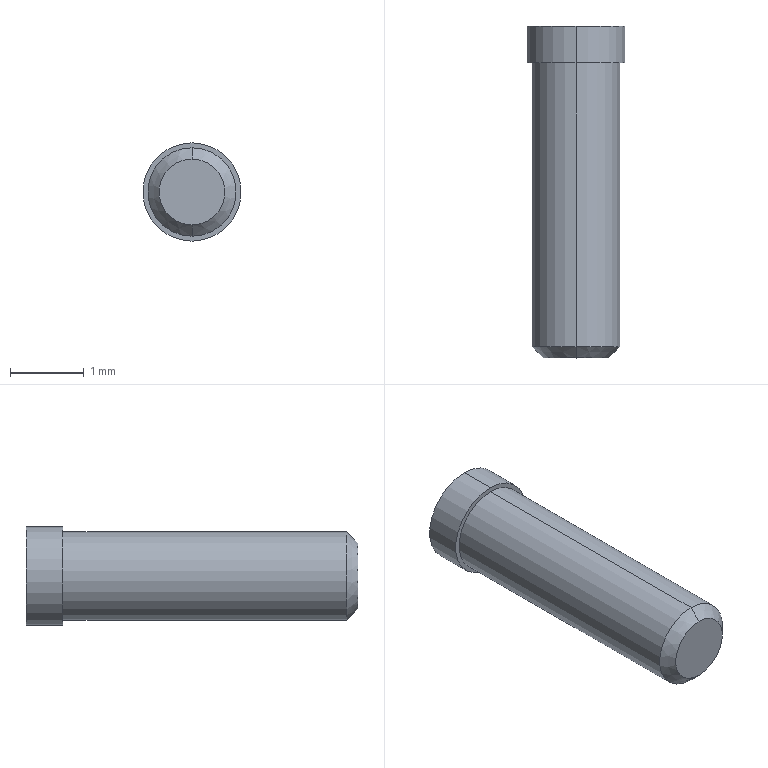Part | STEP file | MG_Plug_Screw_9_N | 1 solid | 16 faces | box 1.333 x 4.5 x 1.333 mm | volume 5.052 mm3 | plane 10 | cylinder 4 | cone 2 | commonest cylinder face diameters 1.2 x2 1.333 x2
STEP:
#1=CARTESIAN_POINT('',(0.,0.,0.));
#2=DIRECTION('',(0.,0.,1.));
#3=DIRECTION('',(1.,0.,0.));
#4=AXIS2_PLACEMENT_3D('',#1,#2,#3);
#5=CARTESIAN_POINT('',(0.,-4.,0.4465));
#6=VERTEX_POINT('',#5);
#7=CARTESIAN_POINT('',(0.,-4.,-0.4465));
#8=VERTEX_POINT('',#7);
#9=CARTESIAN_POINT('',(0.,-4.,0.));
#10=DIRECTION('',(0.,1.,0.));
#11=DIRECTION('',(0.,0.,1.));
#12=AXIS2_PLACEMENT_3D('',#9,#10,#11);
#13=CIRCLE('',#12,0.4465);
#14=CARTESIAN_POINT('',(0.,-4.,0.));
#15=DIRECTION('',(0.,1.,0.));
#16=DIRECTION('',(0.,0.,1.));
#17=AXIS2_PLACEMENT_3D('',#14,#15,#16);
#18=CONICAL_SURFACE('',#17,0.4465,0.7854);
#19=CARTESIAN_POINT('',(0.,0.));
#20=DIRECTION('',(1.,0.));
#21=VECTOR('',#20,1.);
#22=LINE('',#19,#21);
#23=(GEOMETRIC_REPRESENTATION_CONTEXT(2)PARAMETRIC_REPRESENTATION_CONTEXT()REPRESENTATION_CONTEXT('',''));
#24=DEFINITIONAL_REPRESENTATION('',(#22),#23);
#25=PCURVE('',#18,#24);
#26=CARTESIAN_POINT('',(0.4465,-4.,0.));
#27=DIRECTION('',(0.,1.,0.));
#28=DIRECTION('',(0.,0.,1.));
#29=AXIS2_PLACEMENT_3D('',#26,#27,#28);
#30=PLANE('',#29);
#31=CARTESIAN_POINT('',(0.,-0.4465));
#32=DIRECTION('',(1.,0.));
#33=AXIS2_PLACEMENT_2D('',#31,#32);
#34=CIRCLE('',#33,0.4465);
#35=(GEOMETRIC_REPRESENTATION_CONTEXT(2)PARAMETRIC_REPRESENTATION_CONTEXT()REPRESENTATION_CONTEXT('',''));
#36=DEFINITIONAL_REPRESENTATION('',(#34),#35);
#37=PCURVE('',#30,#36);
#38=SURFACE_CURVE('',#13,(#25,#37),.PCURVE_S1.);
#39=EDGE_CURVE('',#6,#8,#38,.T.);
#40=ORIENTED_EDGE('',*,*,#39,.T.);
#41=CARTESIAN_POINT('',(0.,-3.846,-0.6));
#42=VERTEX_POINT('',#41);
#43=CARTESIAN_POINT('',(0.,-4.,-0.4465));
#44=DIRECTION('',(0.,0.7071,-0.7071));
#45=VECTOR('',#44,1.);
#46=LINE('',#43,#45);
#47=CARTESIAN_POINT('',(3.142,0.));
#48=DIRECTION('',(0.,1.));
#49=VECTOR('',#48,1.);
#50=LINE('',#47,#49);
#51=(GEOMETRIC_REPRESENTATION_CONTEXT(2)PARAMETRIC_REPRESENTATION_CONTEXT()REPRESENTATION_CONTEXT('',''));
#52=DEFINITIONAL_REPRESENTATION('',(#50),#51);
#53=PCURVE('',#18,#52);
#54=CARTESIAN_POINT('',(0.,-4.,0.));
#55=DIRECTION('',(0.,1.,0.));
#56=DIRECTION('',(0.,0.,1.));
#57=AXIS2_PLACEMENT_3D('',#54,#55,#56);
#58=CONICAL_SURFACE('',#57,0.4465,0.7854);
#59=CARTESIAN_POINT('',(3.142,0.));
#60=DIRECTION('',(0.,1.));
#61=VECTOR('',#60,1.);
#62=LINE('',#59,#61);
#63=(GEOMETRIC_REPRESENTATION_CONTEXT(2)PARAMETRIC_REPRESENTATION_CONTEXT()REPRESENTATION_CONTEXT('',''));
#64=DEFINITIONAL_REPRESENTATION('',(#62),#63);
#65=PCURVE('',#58,#64);
#66=SURFACE_CURVE('',#46,(#53,#65),.PCURVE_S1.);
#67=EDGE_CURVE('',#8,#42,#66,.T.);
#68=ORIENTED_EDGE('',*,*,#67,.T.);
#69=CARTESIAN_POINT('',(0.,-3.846,0.6));
#70=VERTEX_POINT('',#69);
#71=CARTESIAN_POINT('',(0.,-3.846,0.));
#72=DIRECTION('',(0.,1.,0.));
#73=DIRECTION('',(0.,0.,1.));
#74=AXIS2_PLACEMENT_3D('',#71,#72,#73);
#75=CIRCLE('',#74,0.6);
#76=CARTESIAN_POINT('',(0.,0.1535));
#77=DIRECTION('',(1.,0.));
#78=VECTOR('',#77,1.);
#79=LINE('',#76,#78);
#80=(GEOMETRIC_REPRESENTATION_CONTEXT(2)PARAMETRIC_REPRESENTATION_CONTEXT()REPRESENTATION_CONTEXT('',''));
#81=DEFINITIONAL_REPRESENTATION('',(#79),#80);
#82=PCURVE('',#18,#81);
#83=CARTESIAN_POINT('',(0.,-4.,0.));
#84=DIRECTION('',(0.,1.,0.));
#85=DIRECTION('',(0.,0.,1.));
#86=AXIS2_PLACEMENT_3D('',#83,#84,#85);
#87=CYLINDRICAL_SURFACE('',#86,0.6);
#88=CARTESIAN_POINT('',(0.,0.1535));
#89=DIRECTION('',(1.,0.));
#90=VECTOR('',#89,1.);
#91=LINE('',#88,#90);
#92=(GEOMETRIC_REPRESENTATION_CONTEXT(2)PARAMETRIC_REPRESENTATION_CONTEXT()REPRESENTATION_CONTEXT('',''));
#93=DEFINITIONAL_REPRESENTATION('',(#91),#92);
#94=PCURVE('',#87,#93);
#95=SURFACE_CURVE('',#75,(#82,#94),.PCURVE_S1.);
#96=EDGE_CURVE('',#70,#42,#95,.T.);
#97=ORIENTED_EDGE('',*,*,#96,.F.);
#98=CARTESIAN_POINT('',(0.,-4.,0.4465));
#99=DIRECTION('',(0.,0.7071,0.7071));
#100=VECTOR('',#99,1.);
#101=LINE('',#98,#100);
#102=CARTESIAN_POINT('',(0.,0.));
#103=DIRECTION('',(0.,1.));
#104=VECTOR('',#103,1.);
#105=LINE('',#102,#104);
#106=(GEOMETRIC_REPRESENTATION_CONTEXT(2)PARAMETRIC_REPRESENTATION_CONTEXT()REPRESENTATION_CONTEXT('',''));
#107=DEFINITIONAL_REPRESENTATION('',(#105),#106);
#108=PCURVE('',#18,#107);
#109=CARTESIAN_POINT('',(6.283,0.));
#110=DIRECTION('',(0.,1.));
#111=VECTOR('',#110,1.);
#112=LINE('',#109,#111);
#113=(GEOMETRIC_REPRESENTATION_CONTEXT(2)PARAMETRIC_REPRESENTATION_CONTEXT()REPRESENTATION_CONTEXT('',''));
#114=DEFINITIONAL_REPRESENTATION('',(#112),#113);
#115=PCURVE('',#58,#114);
#116=SURFACE_CURVE('',#101,(#108,#115),.PCURVE_S1.);
#117=EDGE_CURVE('',#6,#70,#116,.T.);
#118=ORIENTED_EDGE('',*,*,#117,.F.);
#119=EDGE_LOOP('',(#40,#68,#97,#118));
#120=FACE_BOUND('',#119,.T.);
#121=ADVANCED_FACE('',(#120),#18,.T.);
#122=ORIENTED_EDGE('',*,*,#96,.T.);
#123=CARTESIAN_POINT('',(0.,0.,-0.6));
#124=VERTEX_POINT('',#123);
#125=CARTESIAN_POINT('',(0.,-4.,-0.6));
#126=DIRECTION('',(0.,1.,0.));
#127=VECTOR('',#126,1.);
#128=LINE('',#125,#127);
#129=CARTESIAN_POINT('',(3.142,0.));
#130=DIRECTION('',(0.,1.));
#131=VECTOR('',#130,1.);
#132=LINE('',#129,#131);
#133=(GEOMETRIC_REPRESENTATION_CONTEXT(2)PARAMETRIC_REPRESENTATION_CONTEXT()REPRESENTATION_CONTEXT('',''));
#134=DEFINITIONAL_REPRESENTATION('',(#132),#133);
#135=PCURVE('',#87,#134);
#136=CARTESIAN_POINT('',(0.,-4.,0.));
#137=DIRECTION('',(0.,1.,0.));
#138=DIRECTION('',(0.,0.,1.));
#139=AXIS2_PLACEMENT_3D('',#136,#137,#138);
#140=CYLINDRICAL_SURFACE('',#139,0.6);
#141=CARTESIAN_POINT('',(3.142,0.));
#142=DIRECTION('',(0.,1.));
#143=VECTOR('',#142,1.);
#144=LINE('',#141,#143);
#145=(GEOMETRIC_REPRESENTATION_CONTEXT(2)PARAMETRIC_REPRESENTATION_CONTEXT()REPRESENTATION_CONTEXT('',''));
#146=DEFINITIONAL_REPRESENTATION('',(#144),#145);
#147=PCURVE('',#140,#146);
#148=SURFACE_CURVE('',#128,(#135,#147),.PCURVE_S1.);
#149=EDGE_CURVE('',#42,#124,#148,.T.);
#150=ORIENTED_EDGE('',*,*,#149,.T.);
#151=CARTESIAN_POINT('',(0.,0.,0.6));
#152=VERTEX_POINT('',#151);
#153=CARTESIAN_POINT('',(0.,0.,0.));
#154=DIRECTION('',(0.,1.,0.));
#155=DIRECTION('',(0.,0.,1.));
#156=AXIS2_PLACEMENT_3D('',#153,#154,#155);
#157=CIRCLE('',#156,0.6);
#158=CARTESIAN_POINT('',(0.,4.));
#159=DIRECTION('',(1.,0.));
#160=VECTOR('',#159,1.);
#161=LINE('',#158,#160);
#162=(GEOMETRIC_REPRESENTATION_CONTEXT(2)PARAMETRIC_REPRESENTATION_CONTEXT()REPRESENTATION_CONTEXT('',''));
#163=DEFINITIONAL_REPRESENTATION('',(#161),#162);
#164=PCURVE('',#87,#163);
#165=CARTESIAN_POINT('',(0.6667,0.,0.));
#166=DIRECTION('',(0.,1.,0.));
#167=DIRECTION('',(0.,0.,1.));
#168=AXIS2_PLACEMENT_3D('',#165,#166,#167);
#169=PLANE('',#168);
#170=CARTESIAN_POINT('',(0.,-0.6667));
#171=DIRECTION('',(1.,0.));
#172=AXIS2_PLACEMENT_2D('',#170,#171);
#173=CIRCLE('',#172,0.6);
#174=(GEOMETRIC_REPRESENTATION_CONTEXT(2)PARAMETRIC_REPRESENTATION_CONTEXT()REPRESENTATION_CONTEXT('',''));
#175=DEFINITIONAL_REPRESENTATION('',(#173),#174);
#176=PCURVE('',#169,#175);
#177=SURFACE_CURVE('',#157,(#164,#176),.PCURVE_S1.);
#178=EDGE_CURVE('',#152,#124,#177,.T.);
#179=ORIENTED_EDGE('',*,*,#178,.F.);
#180=CARTESIAN_POINT('',(0.,-4.,0.6));
#181=DIRECTION('',(0.,1.,0.));
#182=VECTOR('',#181,1.);
#183=LINE('',#180,#182);
#184=CARTESIAN_POINT('',(0.,0.));
#185=DIRECTION('',(0.,1.));
#186=VECTOR('',#185,1.);
#187=LINE('',#184,#186);
#188=(GEOMETRIC_REPRESENTATION_CONTEXT(2)PARAMETRIC_REPRESENTATION_CONTEXT()REPRESENTATION_CONTEXT('',''));
#189=DEFINITIONAL_REPRESENTATION('',(#187),#188);
#190=PCURVE('',#87,#189);
#191=CARTESIAN_POINT('',(6.283,0.));
#192=DIRECTION('',(0.,1.));
#193=VECTOR('',#192,1.);
#194=LINE('',#191,#193);
#195=(GEOMETRIC_REPRESENTATION_CONTEXT(2)PARAMETRIC_REPRESENTATION_CONTEXT()REPRESENTATION_CONTEXT('',''));
#196=DEFINITIONAL_REPRESENTATION('',(#194),#195);
#197=PCURVE('',#140,#196);
#198=SURFACE_CURVE('',#183,(#190,#197),.PCURVE_S1.);
#199=EDGE_CURVE('',#70,#152,#198,.T.);
#200=ORIENTED_EDGE('',*,*,#199,.F.);
#201=EDGE_LOOP('',(#122,#150,#179,#200));
#202=FACE_BOUND('',#201,.T.);
#203=ADVANCED_FACE('',(#202),#87,.T.);
#204=CARTESIAN_POINT('',(0.,0.,0.6667));
#205=VERTEX_POINT('',#204);
#206=CARTESIAN_POINT('',(0.,0.,-0.6667));
#207=VERTEX_POINT('',#206);
#208=CARTESIAN_POINT('',(0.,0.,0.));
#209=DIRECTION('',(0.,1.,0.));
#210=DIRECTION('',(0.,0.,1.));
#211=AXIS2_PLACEMENT_3D('',#208,#209,#210);
#212=CIRCLE('',#211,0.6667);
#213=CARTESIAN_POINT('',(0.,-4.,0.));
#214=DIRECTION('',(0.,1.,0.));
#215=DIRECTION('',(0.,0.,1.));
#216=AXIS2_PLACEMENT_3D('',#213,#214,#215);
#217=CYLINDRICAL_SURFACE('',#216,0.6667);
#218=CARTESIAN_POINT('',(0.,4.));
#219=DIRECTION('',(1.,0.));
#220=VECTOR('',#219,1.);
#221=LINE('',#218,#220);
#222=(GEOMETRIC_REPRESENTATION_CONTEXT(2)PARAMETRIC_REPRESENTATION_CONTEXT()REPRESENTATION_CONTEXT('',''));
#223=DEFINITIONAL_REPRESENTATION('',(#221),#222);
#224=PCURVE('',#217,#223);
#225=CARTESIAN_POINT('',(0.,-0.6667));
#226=DIRECTION('',(1.,0.));
#227=AXIS2_PLACEMENT_2D('',#225,#226);
#228=CIRCLE('',#227,0.6667);
#229=(GEOMETRIC_REPRESENTATION_CONTEXT(2)PARAMETRIC_REPRESENTATION_CONTEXT()REPRESENTATION_CONTEXT('',''));
#230=DEFINITIONAL_REPRESENTATION('',(#228),#229);
#231=PCURVE('',#169,#230);
#232=SURFACE_CURVE('',#212,(#224,#231),.PCURVE_S1.);
#233=EDGE_CURVE('',#205,#207,#232,.T.);
#234=ORIENTED_EDGE('',*,*,#233,.T.);
#235=CARTESIAN_POINT('',(0.,0.5,-0.6667));
#236=VERTEX_POINT('',#235);
#237=CARTESIAN_POINT('',(0.,-4.,-0.6667));
#238=DIRECTION('',(0.,1.,0.));
#239=VECTOR('',#238,1.);
#240=LINE('',#237,#239);
#241=CARTESIAN_POINT('',(3.142,0.));
#242=DIRECTION('',(0.,1.));
#243=VECTOR('',#242,1.);
#244=LINE('',#241,#243);
#245=(GEOMETRIC_REPRESENTATION_CONTEXT(2)PARAMETRIC_REPRESENTATION_CONTEXT()REPRESENTATION_CONTEXT('',''));
#246=DEFINITIONAL_REPRESENTATION('',(#244),#245);
#247=PCURVE('',#217,#246);
#248=CARTESIAN_POINT('',(0.,-4.,0.));
#249=DIRECTION('',(0.,1.,0.));
#250=DIRECTION('',(0.,0.,1.));
#251=AXIS2_PLACEMENT_3D('',#248,#249,#250);
#252=CYLINDRICAL_SURFACE('',#251,0.6667);
#253=CARTESIAN_POINT('',(3.142,0.));
#254=DIRECTION('',(0.,1.));
#255=VECTOR('',#254,1.);
#256=LINE('',#253,#255);
#257=(GEOMETRIC_REPRESENTATION_CONTEXT(2)PARAMETRIC_REPRESENTATION_CONTEXT()REPRESENTATION_CONTEXT('',''));
#258=DEFINITIONAL_REPRESENTATION('',(#256),#257);
#259=PCURVE('',#252,#258);
#260=SURFACE_CURVE('',#240,(#247,#259),.PCURVE_S1.);
#261=EDGE_CURVE('',#207,#236,#260,.T.);
#262=ORIENTED_EDGE('',*,*,#261,.T.);
#263=CARTESIAN_POINT('',(0.,0.5,0.6667));
#264=VERTEX_POINT('',#263);
#265=CARTESIAN_POINT('',(0.,0.5,0.));
#266=DIRECTION('',(0.,1.,0.));
#267=DIRECTION('',(0.,0.,1.));
#268=AXIS2_PLACEMENT_3D('',#265,#266,#267);
#269=CIRCLE('',#268,0.6667);
#270=CARTESIAN_POINT('',(0.,4.5));
#271=DIRECTION('',(1.,0.));
#272=VECTOR('',#271,1.);
#273=LINE('',#270,#272);
#274=(GEOMETRIC_REPRESENTATION_CONTEXT(2)PARAMETRIC_REPRESENTATION_CONTEXT()REPRESENTATION_CONTEXT('',''));
#275=DEFINITIONAL_REPRESENTATION('',(#273),#274);
#276=PCURVE('',#217,#275);
#277=CARTESIAN_POINT('',(0.,0.5,0.));
#278=DIRECTION('',(0.,-1.,0.));
#279=DIRECTION('',(0.,0.,-1.));
#280=AXIS2_PLACEMENT_3D('',#277,#278,#279);
#281=PLANE('',#280);
#282=CARTESIAN_POINT('',(-0.6667,0.));
#283=CARTESIAN_POINT('',(-0.6667,1.155));
#284=CARTESIAN_POINT('',(0.3333,0.5774));
#285=CARTESIAN_POINT('',(1.333,0.));
#286=CARTESIAN_POINT('',(0.3333,-0.5774));
#287=CARTESIAN_POINT('',(-0.6667,-1.155));
#288=CARTESIAN_POINT('',(-0.6667,0.));
#289=(BOUNDED_CURVE()B_SPLINE_CURVE(2,(#282,#283,#284,#285,#286,#287,#288),.UNSPECIFIED.,.T.,.F.)B_SPLINE_CURVE_WITH_KNOTS((1,2,2,2,2,1),(-2.094,0.,2.094,4.189,6.283,8.378),.UNSPECIFIED.)CURVE()GEOMETRIC_REPRESENTATION_ITEM()RATIONAL_B_SPLINE_CURVE((1.,0.5,1.,0.5,1.,0.5,1.))REPRESENTATION_ITEM(''));
#290=(GEOMETRIC_REPRESENTATION_CONTEXT(2)PARAMETRIC_REPRESENTATION_CONTEXT()REPRESENTATION_CONTEXT('',''));
#291=DEFINITIONAL_REPRESENTATION('',(#289),#290);
#292=PCURVE('',#281,#291);
#293=SURFACE_CURVE('',#269,(#276,#292),.PCURVE_S1.);
#294=EDGE_CURVE('',#264,#236,#293,.T.);
#295=ORIENTED_EDGE('',*,*,#294,.F.);
#296=CARTESIAN_POINT('',(0.,-4.,0.6667));
#297=DIRECTION('',(0.,1.,0.));
#298=VECTOR('',#297,1.);
#299=LINE('',#296,#298);
#300=CARTESIAN_POINT('',(0.,0.));
#301=DIRECTION('',(0.,1.));
#302=VECTOR('',#301,1.);
#303=LINE('',#300,#302);
#304=(GEOMETRIC_REPRESENTATION_CONTEXT(2)PARAMETRIC_REPRESENTATION_CONTEXT()REPRESENTATION_CONTEXT('',''));
#305=DEFINITIONAL_REPRESENTATION('',(#303),#304);
#306=PCURVE('',#217,#305);
#307=CARTESIAN_POINT('',(6.283,0.));
#308=DIRECTION('',(0.,1.));
#309=VECTOR('',#308,1.);
#310=LINE('',#307,#309);
#311=(GEOMETRIC_REPRESENTATION_CONTEXT(2)PARAMETRIC_REPRESENTATION_CONTEXT()REPRESENTATION_CONTEXT('',''));
#312=DEFINITIONAL_REPRESENTATION('',(#310),#311);
#313=PCURVE('',#252,#312);
#314=SURFACE_CURVE('',#299,(#306,#313),.PCURVE_S1.);
#315=EDGE_CURVE('',#205,#264,#314,.T.);
#316=ORIENTED_EDGE('',*,*,#315,.F.);
#317=EDGE_LOOP('',(#234,#262,#295,#316));
#318=FACE_BOUND('',#317,.T.);
#319=ADVANCED_FACE('',(#318),#217,.T.);
#320=CARTESIAN_POINT('',(-0.3871,0.5,0.2235));
#321=VERTEX_POINT('',#320);
#322=CARTESIAN_POINT('',(0.,0.5,0.447));
#323=VERTEX_POINT('',#322);
#324=CARTESIAN_POINT('',(-0.3871,0.5,0.2235));
#325=DIRECTION('',(0.866,0.,0.5));
#326=VECTOR('',#325,1.);
#327=LINE('',#324,#326);
#328=CARTESIAN_POINT('',(-0.2235,-0.3871));
#329=DIRECTION('',(-0.5,0.866));
#330=VECTOR('',#329,1.);
#331=LINE('',#328,#330);
#332=(GEOMETRIC_REPRESENTATION_CONTEXT(2)PARAMETRIC_REPRESENTATION_CONTEXT()REPRESENTATION_CONTEXT('',''));
#333=DEFINITIONAL_REPRESENTATION('',(#331),#332);
#334=PCURVE('',#281,#333);
#335=CARTESIAN_POINT('',(-0.3871,0.25,0.2235));
#336=DIRECTION('',(-0.5,0.,0.866));
#337=DIRECTION('',(0.866,0.,0.5));
#338=AXIS2_PLACEMENT_3D('',#335,#336,#337);
#339=PLANE('',#338);
#340=CARTESIAN_POINT('',(0.,0.25));
#341=DIRECTION('',(1.,0.));
#342=VECTOR('',#341,1.);
#343=LINE('',#340,#342);
#344=(GEOMETRIC_REPRESENTATION_CONTEXT(2)PARAMETRIC_REPRESENTATION_CONTEXT()REPRESENTATION_CONTEXT('',''));
#345=DEFINITIONAL_REPRESENTATION('',(#343),#344);
#346=PCURVE('',#339,#345);
#347=SURFACE_CURVE('',#327,(#334,#346),.PCURVE_S1.);
#348=EDGE_CURVE('',#321,#323,#347,.T.);
#349=ORIENTED_EDGE('',*,*,#348,.F.);
#350=CARTESIAN_POINT('',(-0.3871,0.5,-0.2235));
#351=VERTEX_POINT('',#350);
#352=CARTESIAN_POINT('',(-0.3871,0.5,-0.2235));
#353=DIRECTION('',(0.,0.,1.));
#354=VECTOR('',#353,1.);
#355=LINE('',#352,#354);
#356=CARTESIAN_POINT('',(0.2235,-0.3871));
#357=DIRECTION('',(-1.,0.));
#358=VECTOR('',#357,1.);
#359=LINE('',#356,#358);
#360=(GEOMETRIC_REPRESENTATION_CONTEXT(2)PARAMETRIC_REPRESENTATION_CONTEXT()REPRESENTATION_CONTEXT('',''));
#361=DEFINITIONAL_REPRESENTATION('',(#359),#360);
#362=PCURVE('',#281,#361);
#363=CARTESIAN_POINT('',(-0.3871,0.25,-0.2235));
#364=DIRECTION('',(-1.,0.,0.));
#365=DIRECTION('',(0.,0.,1.));
#366=AXIS2_PLACEMENT_3D('',#363,#364,#365);
#367=PLANE('',#366);
#368=CARTESIAN_POINT('',(0.,0.25));
#369=DIRECTION('',(1.,0.));
#370=VECTOR('',#369,1.);
#371=LINE('',#368,#370);
#372=(GEOMETRIC_REPRESENTATION_CONTEXT(2)PARAMETRIC_REPRESENTATION_CONTEXT()REPRESENTATION_CONTEXT('',''));
#373=DEFINITIONAL_REPRESENTATION('',(#371),#372);
#374=PCURVE('',#367,#373);
#375=SURFACE_CURVE('',#355,(#362,#374),.PCURVE_S1.);
#376=EDGE_CURVE('',#351,#321,#375,.T.);
#377=ORIENTED_EDGE('',*,*,#376,.F.);
#378=CARTESIAN_POINT('',(0.,0.5,-0.447));
#379=VERTEX_POINT('',#378);
#380=CARTESIAN_POINT('',(0.,0.5,-0.447));
#381=DIRECTION('',(-0.866,0.,0.5));
#382=VECTOR('',#381,1.);
#383=LINE('',#380,#382);
#384=CARTESIAN_POINT('',(0.447,0.));
#385=DIRECTION('',(-0.5,-0.866));
#386=VECTOR('',#385,1.);
#387=LINE('',#384,#386);
#388=(GEOMETRIC_REPRESENTATION_CONTEXT(2)PARAMETRIC_REPRESENTATION_CONTEXT()REPRESENTATION_CONTEXT('',''));
#389=DEFINITIONAL_REPRESENTATION('',(#387),#388);
#390=PCURVE('',#281,#389);
#391=CARTESIAN_POINT('',(0.,0.25,-0.447));
#392=DIRECTION('',(-0.5,0.,-0.866));
#393=DIRECTION('',(-0.866,0.,0.5));
#394=AXIS2_PLACEMENT_3D('',#391,#392,#393);
#395=PLANE('',#394);
#396=CARTESIAN_POINT('',(0.,0.25));
#397=DIRECTION('',(1.,0.));
#398=VECTOR('',#397,1.);
#399=LINE('',#396,#398);
#400=(GEOMETRIC_REPRESENTATION_CONTEXT(2)PARAMETRIC_REPRESENTATION_CONTEXT()REPRESENTATION_CONTEXT('',''));
#401=DEFINITIONAL_REPRESENTATION('',(#399),#400);
#402=PCURVE('',#395,#401);
#403=SURFACE_CURVE('',#383,(#390,#402),.PCURVE_S1.);
#404=EDGE_CURVE('',#379,#351,#403,.T.);
#405=ORIENTED_EDGE('',*,*,#404,.F.);
#406=CARTESIAN_POINT('',(0.3871,0.5,-0.2235));
#407=VERTEX_POINT('',#406);
#408=CARTESIAN_POINT('',(0.3871,0.5,-0.2235));
#409=DIRECTION('',(-0.866,0.,-0.5));
#410=VECTOR('',#409,1.);
#411=LINE('',#408,#410);
#412=CARTESIAN_POINT('',(0.2235,0.3871));
#413=DIRECTION('',(0.5,-0.866));
#414=VECTOR('',#413,1.);
#415=LINE('',#412,#414);
#416=(GEOMETRIC_REPRESENTATION_CONTEXT(2)PARAMETRIC_REPRESENTATION_CONTEXT()REPRESENTATION_CONTEXT('',''));
#417=DEFINITIONAL_REPRESENTATION('',(#415),#416);
#418=PCURVE('',#281,#417);
#419=CARTESIAN_POINT('',(0.3871,0.25,-0.2235));
#420=DIRECTION('',(0.5,0.,-0.866));
#421=DIRECTION('',(-0.866,0.,-0.5));
#422=AXIS2_PLACEMENT_3D('',#419,#420,#421);
#423=PLANE('',#422);
#424=CARTESIAN_POINT('',(0.,0.25));
#425=DIRECTION('',(1.,0.));
#426=VECTOR('',#425,1.);
#427=LINE('',#424,#426);
#428=(GEOMETRIC_REPRESENTATION_CONTEXT(2)PARAMETRIC_REPRESENTATION_CONTEXT()REPRESENTATION_CONTEXT('',''));
#429=DEFINITIONAL_REPRESENTATION('',(#427),#428);
#430=PCURVE('',#423,#429);
#431=SURFACE_CURVE('',#411,(#418,#430),.PCURVE_S1.);
#432=EDGE_CURVE('',#407,#379,#431,.T.);
#433=ORIENTED_EDGE('',*,*,#432,.F.);
#434=CARTESIAN_POINT('',(0.3871,0.5,0.2235));
#435=VERTEX_POINT('',#434);
#436=CARTESIAN_POINT('',(0.3871,0.5,0.2235));
#437=DIRECTION('',(0.,0.,-1.));
#438=VECTOR('',#437,1.);
#439=LINE('',#436,#438);
#440=CARTESIAN_POINT('',(-0.2235,0.3871));
#441=DIRECTION('',(1.,0.));
#442=VECTOR('',#441,1.);
#443=LINE('',#440,#442);
#444=(GEOMETRIC_REPRESENTATION_CONTEXT(2)PARAMETRIC_REPRESENTATION_CONTEXT()REPRESENTATION_CONTEXT('',''));
#445=DEFINITIONAL_REPRESENTATION('',(#443),#444);
#446=PCURVE('',#281,#445);
#447=CARTESIAN_POINT('',(0.3871,0.25,0.2235));
#448=DIRECTION('',(1.,0.,0.));
#449=DIRECTION('',(0.,0.,-1.));
#450=AXIS2_PLACEMENT_3D('',#447,#448,#449);
#451=PLANE('',#450);
#452=CARTESIAN_POINT('',(0.,0.25));
#453=DIRECTION('',(1.,0.));
#454=VECTOR('',#453,1.);
#455=LINE('',#452,#454);
#456=(GEOMETRIC_REPRESENTATION_CONTEXT(2)PARAMETRIC_REPRESENTATION_CONTEXT()REPRESENTATION_CONTEXT('',''));
#457=DEFINITIONAL_REPRESENTATION('',(#455),#456);
#458=PCURVE('',#451,#457);
#459=SURFACE_CURVE('',#439,(#446,#458),.PCURVE_S1.);
#460=EDGE_CURVE('',#435,#407,#459,.T.);
#461=ORIENTED_EDGE('',*,*,#460,.F.);
#462=CARTESIAN_POINT('',(0.,0.5,0.447));
#463=DIRECTION('',(0.866,0.,-0.5));
#464=VECTOR('',#463,1.);
#465=LINE('',#462,#464);
#466=CARTESIAN_POINT('',(-0.447,0.));
#467=DIRECTION('',(0.5,0.866));
#468=VECTOR('',#467,1.);
#469=LINE('',#466,#468);
#470=(GEOMETRIC_REPRESENTATION_CONTEXT(2)PARAMETRIC_REPRESENTATION_CONTEXT()REPRESENTATION_CONTEXT('',''));
#471=DEFINITIONAL_REPRESENTATION('',(#469),#470);
#472=PCURVE('',#281,#471);
#473=CARTESIAN_POINT('',(0.,0.25,0.447));
#474=DIRECTION('',(0.5,0.,0.866));
#475=DIRECTION('',(0.866,0.,-0.5));
#476=AXIS2_PLACEMENT_3D('',#473,#474,#475);
#477=PLANE('',#476);
#478=CARTESIAN_POINT('',(0.,0.25));
#479=DIRECTION('',(1.,0.));
#480=VECTOR('',#479,1.);
#481=LINE('',#478,#480);
#482=(GEOMETRIC_REPRESENTATION_CONTEXT(2)PARAMETRIC_REPRESENTATION_CONTEXT()REPRESENTATION_CONTEXT('',''));
#483=DEFINITIONAL_REPRESENTATION('',(#481),#482);
#484=PCURVE('',#477,#483);
#485=SURFACE_CURVE('',#465,(#472,#484),.PCURVE_S1.);
#486=EDGE_CURVE('',#323,#435,#485,.T.);
#487=ORIENTED_EDGE('',*,*,#486,.F.);
#488=EDGE_LOOP('',(#349,#377,#405,#433,#461,#487));
#489=FACE_BOUND('',#488,.T.);
#490=ORIENTED_EDGE('',*,*,#294,.T.);
#491=CARTESIAN_POINT('',(0.,0.5,0.));
#492=DIRECTION('',(0.,1.,0.));
#493=DIRECTION('',(0.,0.,1.));
#494=AXIS2_PLACEMENT_3D('',#491,#492,#493);
#495=CIRCLE('',#494,0.6667);
#496=CARTESIAN_POINT('',(-0.6667,0.));
#497=CARTESIAN_POINT('',(-0.6667,1.155));
#498=CARTESIAN_POINT('',(0.3333,0.5774));
#499=CARTESIAN_POINT('',(1.333,0.));
#500=CARTESIAN_POINT('',(0.3333,-0.5774));
#501=CARTESIAN_POINT('',(-0.6667,-1.155));
#502=CARTESIAN_POINT('',(-0.6667,0.));
#503=(BOUNDED_CURVE()B_SPLINE_CURVE(2,(#496,#497,#498,#499,#500,#501,#502),.UNSPECIFIED.,.T.,.F.)B_SPLINE_CURVE_WITH_KNOTS((1,2,2,2,2,1),(-2.094,0.,2.094,4.189,6.283,8.378),.UNSPECIFIED.)CURVE()GEOMETRIC_REPRESENTATION_ITEM()RATIONAL_B_SPLINE_CURVE((1.,0.5,1.,0.5,1.,0.5,1.))REPRESENTATION_ITEM(''));
#504=(GEOMETRIC_REPRESENTATION_CONTEXT(2)PARAMETRIC_REPRESENTATION_CONTEXT()REPRESENTATION_CONTEXT('',''));
#505=DEFINITIONAL_REPRESENTATION('',(#503),#504);
#506=PCURVE('',#281,#505);
#507=CARTESIAN_POINT('',(0.,4.5));
#508=DIRECTION('',(1.,0.));
#509=VECTOR('',#508,1.);
#510=LINE('',#507,#509);
#511=(GEOMETRIC_REPRESENTATION_CONTEXT(2)PARAMETRIC_REPRESENTATION_CONTEXT()REPRESENTATION_CONTEXT('',''));
#512=DEFINITIONAL_REPRESENTATION('',(#510),#511);
#513=PCURVE('',#252,#512);
#514=SURFACE_CURVE('',#495,(#506,#513),.PCURVE_S1.);
#515=EDGE_CURVE('',#236,#264,#514,.T.);
#516=ORIENTED_EDGE('',*,*,#515,.T.);
#517=EDGE_LOOP('',(#490,#516));
#518=FACE_BOUND('',#517,.T.);
#519=ADVANCED_FACE('',(#489,#518),#281,.F.);
#520=ORIENTED_EDGE('',*,*,#261,.F.);
#521=CARTESIAN_POINT('',(0.,0.,0.));
#522=DIRECTION('',(0.,1.,0.));
#523=DIRECTION('',(0.,0.,1.));
#524=AXIS2_PLACEMENT_3D('',#521,#522,#523);
#525=CIRCLE('',#524,0.6667);
#526=CARTESIAN_POINT('',(0.,4.));
#527=DIRECTION('',(1.,0.));
#528=VECTOR('',#527,1.);
#529=LINE('',#526,#528);
#530=(GEOMETRIC_REPRESENTATION_CONTEXT(2)PARAMETRIC_REPRESENTATION_CONTEXT()REPRESENTATION_CONTEXT('',''));
#531=DEFINITIONAL_REPRESENTATION('',(#529),#530);
#532=PCURVE('',#252,#531);
#533=CARTESIAN_POINT('',(0.,-0.6667));
#534=DIRECTION('',(1.,0.));
#535=AXIS2_PLACEMENT_2D('',#533,#534);
#536=CIRCLE('',#535,0.6667);
#537=(GEOMETRIC_REPRESENTATION_CONTEXT(2)PARAMETRIC_REPRESENTATION_CONTEXT()REPRESENTATION_CONTEXT('',''));
#538=DEFINITIONAL_REPRESENTATION('',(#536),#537);
#539=PCURVE('',#169,#538);
#540=SURFACE_CURVE('',#525,(#532,#539),.PCURVE_S1.);
#541=EDGE_CURVE('',#207,#205,#540,.T.);
#542=ORIENTED_EDGE('',*,*,#541,.T.);
#543=ORIENTED_EDGE('',*,*,#315,.T.);
#544=ORIENTED_EDGE('',*,*,#515,.F.);
#545=EDGE_LOOP('',(#520,#542,#543,#544));
#546=FACE_BOUND('',#545,.T.);
#547=ADVANCED_FACE('',(#546),#252,.T.);
#548=ORIENTED_EDGE('',*,*,#233,.F.);
#549=ORIENTED_EDGE('',*,*,#541,.F.);
#550=EDGE_LOOP('',(#548,#549));
#551=FACE_BOUND('',#550,.T.);
#552=ORIENTED_EDGE('',*,*,#178,.T.);
#553=CARTESIAN_POINT('',(0.,0.,0.));
#554=DIRECTION('',(0.,1.,0.));
#555=DIRECTION('',(0.,0.,1.));
#556=AXIS2_PLACEMENT_3D('',#553,#554,#555);
#557=CIRCLE('',#556,0.6);
#558=CARTESIAN_POINT('',(0.,-0.6667));
#559=DIRECTION('',(1.,0.));
#560=AXIS2_PLACEMENT_2D('',#558,#559);
#561=CIRCLE('',#560,0.6);
#562=(GEOMETRIC_REPRESENTATION_CONTEXT(2)PARAMETRIC_REPRESENTATION_CONTEXT()REPRESENTATION_CONTEXT('',''));
#563=DEFINITIONAL_REPRESENTATION('',(#561),#562);
#564=PCURVE('',#169,#563);
#565=CARTESIAN_POINT('',(0.,4.));
#566=DIRECTION('',(1.,0.));
#567=VECTOR('',#566,1.);
#568=LINE('',#565,#567);
#569=(GEOMETRIC_REPRESENTATION_CONTEXT(2)PARAMETRIC_REPRESENTATION_CONTEXT()REPRESENTATION_CONTEXT('',''));
#570=DEFINITIONAL_REPRESENTATION('',(#568),#569);
#571=PCURVE('',#140,#570);
#572=SURFACE_CURVE('',#557,(#564,#571),.PCURVE_S1.);
#573=EDGE_CURVE('',#124,#152,#572,.T.);
#574=ORIENTED_EDGE('',*,*,#573,.T.);
#575=EDGE_LOOP('',(#552,#574));
#576=FACE_BOUND('',#575,.T.);
#577=ADVANCED_FACE('',(#551,#576),#169,.F.);
#578=ORIENTED_EDGE('',*,*,#149,.F.);
#579=CARTESIAN_POINT('',(0.,-3.846,0.));
#580=DIRECTION('',(0.,1.,0.));
#581=DIRECTION('',(0.,0.,1.));
#582=AXIS2_PLACEMENT_3D('',#579,#580,#581);
#583=CIRCLE('',#582,0.6);
#584=CARTESIAN_POINT('',(0.,0.1535));
#585=DIRECTION('',(1.,0.));
#586=VECTOR('',#585,1.);
#587=LINE('',#584,#586);
#588=(GEOMETRIC_REPRESENTATION_CONTEXT(2)PARAMETRIC_REPRESENTATION_CONTEXT()REPRESENTATION_CONTEXT('',''));
#589=DEFINITIONAL_REPRESENTATION('',(#587),#588);
#590=PCURVE('',#140,#589);
#591=CARTESIAN_POINT('',(0.,0.1535));
#592=DIRECTION('',(1.,0.));
#593=VECTOR('',#592,1.);
#594=LINE('',#591,#593);
#595=(GEOMETRIC_REPRESENTATION_CONTEXT(2)PARAMETRIC_REPRESENTATION_CONTEXT()REPRESENTATION_CONTEXT('',''));
#596=DEFINITIONAL_REPRESENTATION('',(#594),#595);
#597=PCURVE('',#58,#596);
#598=SURFACE_CURVE('',#583,(#590,#597),.PCURVE_S1.);
#599=EDGE_CURVE('',#42,#70,#598,.T.);
#600=ORIENTED_EDGE('',*,*,#599,.T.);
#601=ORIENTED_EDGE('',*,*,#199,.T.);
#602=ORIENTED_EDGE('',*,*,#573,.F.);
#603=EDGE_LOOP('',(#578,#600,#601,#602));
#604=FACE_BOUND('',#603,.T.);
#605=ADVANCED_FACE('',(#604),#140,.T.);
#606=ORIENTED_EDGE('',*,*,#67,.F.);
#607=CARTESIAN_POINT('',(0.,-4.,0.));
#608=DIRECTION('',(0.,1.,0.));
#609=DIRECTION('',(0.,0.,1.));
#610=AXIS2_PLACEMENT_3D('',#607,#608,#609);
#611=CIRCLE('',#610,0.4465);
#612=CARTESIAN_POINT('',(0.,0.));
#613=DIRECTION('',(1.,0.));
#614=VECTOR('',#613,1.);
#615=LINE('',#612,#614);
#616=(GEOMETRIC_REPRESENTATION_CONTEXT(2)PARAMETRIC_REPRESENTATION_CONTEXT()REPRESENTATION_CONTEXT('',''));
#617=DEFINITIONAL_REPRESENTATION('',(#615),#616);
#618=PCURVE('',#58,#617);
#619=CARTESIAN_POINT('',(0.,-0.4465));
#620=DIRECTION('',(1.,0.));
#621=AXIS2_PLACEMENT_2D('',#619,#620);
#622=CIRCLE('',#621,0.4465);
#623=(GEOMETRIC_REPRESENTATION_CONTEXT(2)PARAMETRIC_REPRESENTATION_CONTEXT()REPRESENTATION_CONTEXT('',''));
#624=DEFINITIONAL_REPRESENTATION('',(#622),#623);
#625=PCURVE('',#30,#624);
#626=SURFACE_CURVE('',#611,(#618,#625),.PCURVE_S1.);
#627=EDGE_CURVE('',#8,#6,#626,.T.);
#628=ORIENTED_EDGE('',*,*,#627,.T.);
#629=ORIENTED_EDGE('',*,*,#117,.T.);
#630=ORIENTED_EDGE('',*,*,#599,.F.);
#631=EDGE_LOOP('',(#606,#628,#629,#630));
#632=FACE_BOUND('',#631,.T.);
#633=ADVANCED_FACE('',(#632),#58,.T.);
#634=ORIENTED_EDGE('',*,*,#39,.F.);
#635=ORIENTED_EDGE('',*,*,#627,.F.);
#636=EDGE_LOOP('',(#634,#635));
#637=FACE_BOUND('',#636,.T.);
#638=ADVANCED_FACE('',(#637),#30,.F.);
#639=ORIENTED_EDGE('',*,*,#376,.T.);
#640=CARTESIAN_POINT('',(-0.3871,0.25,0.2235));
#641=VERTEX_POINT('',#640);
#642=CARTESIAN_POINT('',(-0.3871,0.25,0.2235));
#643=DIRECTION('',(0.,1.,0.));
#644=VECTOR('',#643,1.);
#645=LINE('',#642,#644);
#646=CARTESIAN_POINT('',(0.447,0.));
#647=DIRECTION('',(0.,1.));
#648=VECTOR('',#647,1.);
#649=LINE('',#646,#648);
#650=(GEOMETRIC_REPRESENTATION_CONTEXT(2)PARAMETRIC_REPRESENTATION_CONTEXT()REPRESENTATION_CONTEXT('',''));
#651=DEFINITIONAL_REPRESENTATION('',(#649),#650);
#652=PCURVE('',#367,#651);
#653=CARTESIAN_POINT('',(0.,0.));
#654=DIRECTION('',(0.,1.));
#655=VECTOR('',#654,1.);
#656=LINE('',#653,#655);
#657=(GEOMETRIC_REPRESENTATION_CONTEXT(2)PARAMETRIC_REPRESENTATION_CONTEXT()REPRESENTATION_CONTEXT('',''));
#658=DEFINITIONAL_REPRESENTATION('',(#656),#657);
#659=PCURVE('',#339,#658);
#660=SURFACE_CURVE('',#645,(#652,#659),.PCURVE_S1.);
#661=EDGE_CURVE('',#641,#321,#660,.T.);
#662=ORIENTED_EDGE('',*,*,#661,.F.);
#663=CARTESIAN_POINT('',(-0.3871,0.25,-0.2235));
#664=VERTEX_POINT('',#663);
#665=CARTESIAN_POINT('',(-0.3871,0.25,-0.2235));
#666=DIRECTION('',(0.,0.,1.));
#667=VECTOR('',#666,1.);
#668=LINE('',#665,#667);
#669=CARTESIAN_POINT('',(0.,0.));
#670=DIRECTION('',(1.,0.));
#671=VECTOR('',#670,1.);
#672=LINE('',#669,#671);
#673=(GEOMETRIC_REPRESENTATION_CONTEXT(2)PARAMETRIC_REPRESENTATION_CONTEXT()REPRESENTATION_CONTEXT('',''));
#674=DEFINITIONAL_REPRESENTATION('',(#672),#673);
#675=PCURVE('',#367,#674);
#676=CARTESIAN_POINT('',(0.,0.25,0.));
#677=DIRECTION('',(0.,1.,0.));
#678=DIRECTION('',(0.,0.,1.));
#679=AXIS2_PLACEMENT_3D('',#676,#677,#678);
#680=PLANE('',#679);
#681=CARTESIAN_POINT('',(-0.2235,-0.3871));
#682=DIRECTION('',(1.,0.));
#683=VECTOR('',#682,1.);
#684=LINE('',#681,#683);
#685=(GEOMETRIC_REPRESENTATION_CONTEXT(2)PARAMETRIC_REPRESENTATION_CONTEXT()REPRESENTATION_CONTEXT('',''));
#686=DEFINITIONAL_REPRESENTATION('',(#684),#685);
#687=PCURVE('',#680,#686);
#688=SURFACE_CURVE('',#668,(#675,#687),.PCURVE_S1.);
#689=EDGE_CURVE('',#664,#641,#688,.T.);
#690=ORIENTED_EDGE('',*,*,#689,.F.);
#691=CARTESIAN_POINT('',(-0.3871,0.25,-0.2235));
#692=DIRECTION('',(0.,1.,0.));
#693=VECTOR('',#692,1.);
#694=LINE('',#691,#693);
#695=CARTESIAN_POINT('',(0.,0.));
#696=DIRECTION('',(0.,1.));
#697=VECTOR('',#696,1.);
#698=LINE('',#695,#697);
#699=(GEOMETRIC_REPRESENTATION_CONTEXT(2)PARAMETRIC_REPRESENTATION_CONTEXT()REPRESENTATION_CONTEXT('',''));
#700=DEFINITIONAL_REPRESENTATION('',(#698),#699);
#701=PCURVE('',#367,#700);
#702=CARTESIAN_POINT('',(0.447,0.));
#703=DIRECTION('',(0.,1.));
#704=VECTOR('',#703,1.);
#705=LINE('',#702,#704);
#706=(GEOMETRIC_REPRESENTATION_CONTEXT(2)PARAMETRIC_REPRESENTATION_CONTEXT()REPRESENTATION_CONTEXT('',''));
#707=DEFINITIONAL_REPRESENTATION('',(#705),#706);
#708=PCURVE('',#395,#707);
#709=SURFACE_CURVE('',#694,(#701,#708),.PCURVE_S1.);
#710=EDGE_CURVE('',#664,#351,#709,.T.);
#711=ORIENTED_EDGE('',*,*,#710,.T.);
#712=EDGE_LOOP('',(#639,#662,#690,#711));
#713=FACE_BOUND('',#712,.T.);
#714=ADVANCED_FACE('',(#713),#367,.F.);
#715=ORIENTED_EDGE('',*,*,#404,.T.);
#716=ORIENTED_EDGE('',*,*,#710,.F.);
#717=CARTESIAN_POINT('',(0.,0.25,-0.447));
#718=VERTEX_POINT('',#717);
#719=CARTESIAN_POINT('',(0.,0.25,-0.447));
#720=DIRECTION('',(-0.866,0.,0.5));
#721=VECTOR('',#720,1.);
#722=LINE('',#719,#721);
#723=CARTESIAN_POINT('',(0.,0.));
#724=DIRECTION('',(1.,0.));
#725=VECTOR('',#724,1.);
#726=LINE('',#723,#725);
#727=(GEOMETRIC_REPRESENTATION_CONTEXT(2)PARAMETRIC_REPRESENTATION_CONTEXT()REPRESENTATION_CONTEXT('',''));
#728=DEFINITIONAL_REPRESENTATION('',(#726),#727);
#729=PCURVE('',#395,#728);
#730=CARTESIAN_POINT('',(-0.447,0.));
#731=DIRECTION('',(0.5,-0.866));
#732=VECTOR('',#731,1.);
#733=LINE('',#730,#732);
#734=(GEOMETRIC_REPRESENTATION_CONTEXT(2)PARAMETRIC_REPRESENTATION_CONTEXT()REPRESENTATION_CONTEXT('',''));
#735=DEFINITIONAL_REPRESENTATION('',(#733),#734);
#736=PCURVE('',#680,#735);
#737=SURFACE_CURVE('',#722,(#729,#736),.PCURVE_S1.);
#738=EDGE_CURVE('',#718,#664,#737,.T.);
#739=ORIENTED_EDGE('',*,*,#738,.F.);
#740=CARTESIAN_POINT('',(0.,0.25,-0.447));
#741=DIRECTION('',(0.,1.,0.));
#742=VECTOR('',#741,1.);
#743=LINE('',#740,#742);
#744=CARTESIAN_POINT('',(0.,0.));
#745=DIRECTION('',(0.,1.));
#746=VECTOR('',#745,1.);
#747=LINE('',#744,#746);
#748=(GEOMETRIC_REPRESENTATION_CONTEXT(2)PARAMETRIC_REPRESENTATION_CONTEXT()REPRESENTATION_CONTEXT('',''));
#749=DEFINITIONAL_REPRESENTATION('',(#747),#748);
#750=PCURVE('',#395,#749);
#751=CARTESIAN_POINT('',(0.447,0.));
#752=DIRECTION('',(0.,1.));
#753=VECTOR('',#752,1.);
#754=LINE('',#751,#753);
#755=(GEOMETRIC_REPRESENTATION_CONTEXT(2)PARAMETRIC_REPRESENTATION_CONTEXT()REPRESENTATION_CONTEXT('',''));
#756=DEFINITIONAL_REPRESENTATION('',(#754),#755);
#757=PCURVE('',#423,#756);
#758=SURFACE_CURVE('',#743,(#750,#757),.PCURVE_S1.);
#759=EDGE_CURVE('',#718,#379,#758,.T.);
#760=ORIENTED_EDGE('',*,*,#759,.T.);
#761=EDGE_LOOP('',(#715,#716,#739,#760));
#762=FACE_BOUND('',#761,.T.);
#763=ADVANCED_FACE('',(#762),#395,.F.);
#764=ORIENTED_EDGE('',*,*,#432,.T.);
#765=ORIENTED_EDGE('',*,*,#759,.F.);
#766=CARTESIAN_POINT('',(0.3871,0.25,-0.2235));
#767=VERTEX_POINT('',#766);
#768=CARTESIAN_POINT('',(0.3871,0.25,-0.2235));
#769=DIRECTION('',(-0.866,0.,-0.5));
#770=VECTOR('',#769,1.);
#771=LINE('',#768,#770);
#772=CARTESIAN_POINT('',(0.,0.));
#773=DIRECTION('',(1.,0.));
#774=VECTOR('',#773,1.);
#775=LINE('',#772,#774);
#776=(GEOMETRIC_REPRESENTATION_CONTEXT(2)PARAMETRIC_REPRESENTATION_CONTEXT()REPRESENTATION_CONTEXT('',''));
#777=DEFINITIONAL_REPRESENTATION('',(#775),#776);
#778=PCURVE('',#423,#777);
#779=CARTESIAN_POINT('',(-0.2235,0.3871));
#780=DIRECTION('',(-0.5,-0.866));
#781=VECTOR('',#780,1.);
#782=LINE('',#779,#781);
#783=(GEOMETRIC_REPRESENTATION_CONTEXT(2)PARAMETRIC_REPRESENTATION_CONTEXT()REPRESENTATION_CONTEXT('',''));
#784=DEFINITIONAL_REPRESENTATION('',(#782),#783);
#785=PCURVE('',#680,#784);
#786=SURFACE_CURVE('',#771,(#778,#785),.PCURVE_S1.);
#787=EDGE_CURVE('',#767,#718,#786,.T.);
#788=ORIENTED_EDGE('',*,*,#787,.F.);
#789=CARTESIAN_POINT('',(0.3871,0.25,-0.2235));
#790=DIRECTION('',(0.,1.,0.));
#791=VECTOR('',#790,1.);
#792=LINE('',#789,#791);
#793=CARTESIAN_POINT('',(0.,0.));
#794=DIRECTION('',(0.,1.));
#795=VECTOR('',#794,1.);
#796=LINE('',#793,#795);
#797=(GEOMETRIC_REPRESENTATION_CONTEXT(2)PARAMETRIC_REPRESENTATION_CONTEXT()REPRESENTATION_CONTEXT('',''));
#798=DEFINITIONAL_REPRESENTATION('',(#796),#797);
#799=PCURVE('',#423,#798);
#800=CARTESIAN_POINT('',(0.447,0.));
#801=DIRECTION('',(0.,1.));
#802=VECTOR('',#801,1.);
#803=LINE('',#800,#802);
#804=(GEOMETRIC_REPRESENTATION_CONTEXT(2)PARAMETRIC_REPRESENTATION_CONTEXT()REPRESENTATION_CONTEXT('',''));
#805=DEFINITIONAL_REPRESENTATION('',(#803),#804);
#806=PCURVE('',#451,#805);
#807=SURFACE_CURVE('',#792,(#799,#806),.PCURVE_S1.);
#808=EDGE_CURVE('',#767,#407,#807,.T.);
#809=ORIENTED_EDGE('',*,*,#808,.T.);
#810=EDGE_LOOP('',(#764,#765,#788,#809));
#811=FACE_BOUND('',#810,.T.);
#812=ADVANCED_FACE('',(#811),#423,.F.);
#813=ORIENTED_EDGE('',*,*,#460,.T.);
#814=ORIENTED_EDGE('',*,*,#808,.F.);
#815=CARTESIAN_POINT('',(0.3871,0.25,0.2235));
#816=VERTEX_POINT('',#815);
#817=CARTESIAN_POINT('',(0.3871,0.25,0.2235));
#818=DIRECTION('',(0.,0.,-1.));
#819=VECTOR('',#818,1.);
#820=LINE('',#817,#819);
#821=CARTESIAN_POINT('',(0.,0.));
#822=DIRECTION('',(1.,0.));
#823=VECTOR('',#822,1.);
#824=LINE('',#821,#823);
#825=(GEOMETRIC_REPRESENTATION_CONTEXT(2)PARAMETRIC_REPRESENTATION_CONTEXT()REPRESENTATION_CONTEXT('',''));
#826=DEFINITIONAL_REPRESENTATION('',(#824),#825);
#827=PCURVE('',#451,#826);
#828=CARTESIAN_POINT('',(0.2235,0.3871));
#829=DIRECTION('',(-1.,0.));
#830=VECTOR('',#829,1.);
#831=LINE('',#828,#830);
#832=(GEOMETRIC_REPRESENTATION_CONTEXT(2)PARAMETRIC_REPRESENTATION_CONTEXT()REPRESENTATION_CONTEXT('',''));
#833=DEFINITIONAL_REPRESENTATION('',(#831),#832);
#834=PCURVE('',#680,#833);
#835=SURFACE_CURVE('',#820,(#827,#834),.PCURVE_S1.);
#836=EDGE_CURVE('',#816,#767,#835,.T.);
#837=ORIENTED_EDGE('',*,*,#836,.F.);
#838=CARTESIAN_POINT('',(0.3871,0.25,0.2235));
#839=DIRECTION('',(0.,1.,0.));
#840=VECTOR('',#839,1.);
#841=LINE('',#838,#840);
#842=CARTESIAN_POINT('',(0.,0.));
#843=DIRECTION('',(0.,1.));
#844=VECTOR('',#843,1.);
#845=LINE('',#842,#844);
#846=(GEOMETRIC_REPRESENTATION_CONTEXT(2)PARAMETRIC_REPRESENTATION_CONTEXT()REPRESENTATION_CONTEXT('',''));
#847=DEFINITIONAL_REPRESENTATION('',(#845),#846);
#848=PCURVE('',#451,#847);
#849=CARTESIAN_POINT('',(0.447,0.));
#850=DIRECTION('',(0.,1.));
#851=VECTOR('',#850,1.);
#852=LINE('',#849,#851);
#853=(GEOMETRIC_REPRESENTATION_CONTEXT(2)PARAMETRIC_REPRESENTATION_CONTEXT()REPRESENTATION_CONTEXT('',''));
#854=DEFINITIONAL_REPRESENTATION('',(#852),#853);
#855=PCURVE('',#477,#854);
#856=SURFACE_CURVE('',#841,(#848,#855),.PCURVE_S1.);
#857=EDGE_CURVE('',#816,#435,#856,.T.);
#858=ORIENTED_EDGE('',*,*,#857,.T.);
#859=EDGE_LOOP('',(#813,#814,#837,#858));
#860=FACE_BOUND('',#859,.T.);
#861=ADVANCED_FACE('',(#860),#451,.F.);
#862=ORIENTED_EDGE('',*,*,#486,.T.);
#863=ORIENTED_EDGE('',*,*,#857,.F.);
#864=CARTESIAN_POINT('',(0.,0.25,0.447));
#865=VERTEX_POINT('',#864);
#866=CARTESIAN_POINT('',(0.,0.25,0.447));
#867=DIRECTION('',(0.866,0.,-0.5));
#868=VECTOR('',#867,1.);
#869=LINE('',#866,#868);
#870=CARTESIAN_POINT('',(0.,0.));
#871=DIRECTION('',(1.,0.));
#872=VECTOR('',#871,1.);
#873=LINE('',#870,#872);
#874=(GEOMETRIC_REPRESENTATION_CONTEXT(2)PARAMETRIC_REPRESENTATION_CONTEXT()REPRESENTATION_CONTEXT('',''));
#875=DEFINITIONAL_REPRESENTATION('',(#873),#874);
#876=PCURVE('',#477,#875);
#877=CARTESIAN_POINT('',(0.447,0.));
#878=DIRECTION('',(-0.5,0.866));
#879=VECTOR('',#878,1.);
#880=LINE('',#877,#879);
#881=(GEOMETRIC_REPRESENTATION_CONTEXT(2)PARAMETRIC_REPRESENTATION_CONTEXT()REPRESENTATION_CONTEXT('',''));
#882=DEFINITIONAL_REPRESENTATION('',(#880),#881);
#883=PCURVE('',#680,#882);
#884=SURFACE_CURVE('',#869,(#876,#883),.PCURVE_S1.);
#885=EDGE_CURVE('',#865,#816,#884,.T.);
#886=ORIENTED_EDGE('',*,*,#885,.F.);
#887=CARTESIAN_POINT('',(0.,0.25,0.447));
#888=DIRECTION('',(0.,1.,0.));
#889=VECTOR('',#888,1.);
#890=LINE('',#887,#889);
#891=CARTESIAN_POINT('',(0.,0.));
#892=DIRECTION('',(0.,1.));
#893=VECTOR('',#892,1.);
#894=LINE('',#891,#893);
#895=(GEOMETRIC_REPRESENTATION_CONTEXT(2)PARAMETRIC_REPRESENTATION_CONTEXT()REPRESENTATION_CONTEXT('',''));
#896=DEFINITIONAL_REPRESENTATION('',(#894),#895);
#897=PCURVE('',#477,#896);
#898=CARTESIAN_POINT('',(0.447,0.));
#899=DIRECTION('',(0.,1.));
#900=VECTOR('',#899,1.);
#901=LINE('',#898,#900);
#902=(GEOMETRIC_REPRESENTATION_CONTEXT(2)PARAMETRIC_REPRESENTATION_CONTEXT()REPRESENTATION_CONTEXT('',''));
#903=DEFINITIONAL_REPRESENTATION('',(#901),#902);
#904=PCURVE('',#339,#903);
#905=SURFACE_CURVE('',#890,(#897,#904),.PCURVE_S1.);
#906=EDGE_CURVE('',#865,#323,#905,.T.);
#907=ORIENTED_EDGE('',*,*,#906,.T.);
#908=EDGE_LOOP('',(#862,#863,#886,#907));
#909=FACE_BOUND('',#908,.T.);
#910=ADVANCED_FACE('',(#909),#477,.F.);
#911=ORIENTED_EDGE('',*,*,#348,.T.);
#912=ORIENTED_EDGE('',*,*,#906,.F.);
#913=CARTESIAN_POINT('',(-0.3871,0.25,0.2235));
#914=DIRECTION('',(0.866,0.,0.5));
#915=VECTOR('',#914,1.);
#916=LINE('',#913,#915);
#917=CARTESIAN_POINT('',(0.,0.));
#918=DIRECTION('',(1.,0.));
#919=VECTOR('',#918,1.);
#920=LINE('',#917,#919);
#921=(GEOMETRIC_REPRESENTATION_CONTEXT(2)PARAMETRIC_REPRESENTATION_CONTEXT()REPRESENTATION_CONTEXT('',''));
#922=DEFINITIONAL_REPRESENTATION('',(#920),#921);
#923=PCURVE('',#339,#922);
#924=CARTESIAN_POINT('',(0.2235,-0.3871));
#925=DIRECTION('',(0.5,0.866));
#926=VECTOR('',#925,1.);
#927=LINE('',#924,#926);
#928=(GEOMETRIC_REPRESENTATION_CONTEXT(2)PARAMETRIC_REPRESENTATION_CONTEXT()REPRESENTATION_CONTEXT('',''));
#929=DEFINITIONAL_REPRESENTATION('',(#927),#928);
#930=PCURVE('',#680,#929);
#931=SURFACE_CURVE('',#916,(#923,#930),.PCURVE_S1.);
#932=EDGE_CURVE('',#641,#865,#931,.T.);
#933=ORIENTED_EDGE('',*,*,#932,.F.);
#934=ORIENTED_EDGE('',*,*,#661,.T.);
#935=EDGE_LOOP('',(#911,#912,#933,#934));
#936=FACE_BOUND('',#935,.T.);
#937=ADVANCED_FACE('',(#936),#339,.F.);
#938=ORIENTED_EDGE('',*,*,#689,.T.);
#939=ORIENTED_EDGE('',*,*,#932,.T.);
#940=ORIENTED_EDGE('',*,*,#885,.T.);
#941=ORIENTED_EDGE('',*,*,#836,.T.);
#942=ORIENTED_EDGE('',*,*,#787,.T.);
#943=ORIENTED_EDGE('',*,*,#738,.T.);
#944=EDGE_LOOP('',(#938,#939,#940,#941,#942,#943));
#945=FACE_BOUND('',#944,.T.);
#946=ADVANCED_FACE('',(#945),#680,.T.);
#947=CLOSED_SHELL('',(#121,#203,#319,#519,#547,#577,#605,#633,#638,#714,#763,#812,#861,#910,#937,#946));
#948=MANIFOLD_SOLID_BREP('',#947);
#949=(LENGTH_UNIT()NAMED_UNIT(*)SI_UNIT(.MILLI.,.METRE.));
#950=UNCERTAINTY_MEASURE_WITH_UNIT(LENGTH_MEASURE(0.0000001),#949,'','');
#951=(NAMED_UNIT(*)PLANE_ANGLE_UNIT()SI_UNIT($,.RADIAN.));
#952=(NAMED_UNIT(*)SI_UNIT($,.STERADIAN.)SOLID_ANGLE_UNIT());
#953=(GEOMETRIC_REPRESENTATION_CONTEXT(3)GLOBAL_UNCERTAINTY_ASSIGNED_CONTEXT((#950))GLOBAL_UNIT_ASSIGNED_CONTEXT((#949,#951,#952))REPRESENTATION_CONTEXT('',''));
#954=ADVANCED_BREP_SHAPE_REPRESENTATION('',(#4,#948),#953);